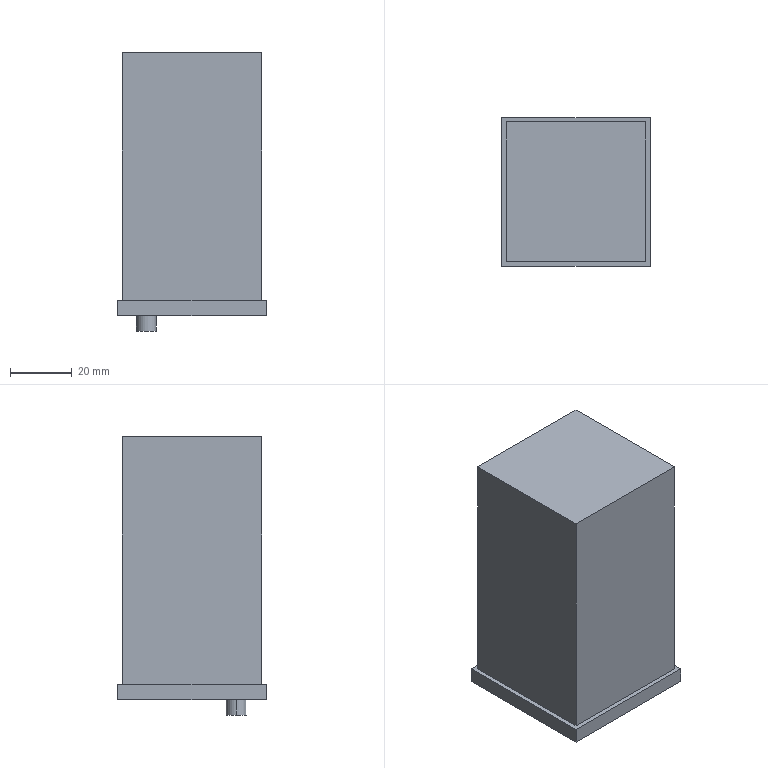Part | STEP file | Magnetic powder tension controller | 1 solid | 19 faces | box 48 x 48 x 90 mm | volume 173670 mm3 | plane 17 | cylinder 2 | commonest cylinder face diameters 6.473 x2
STEP:
#1=CARTESIAN_POINT('',(-17.962,-14.294,-5.));
#2=VERTEX_POINT('',#1);
#3=CARTESIAN_POINT('',(-11.489,-14.294,-5.));
#4=VERTEX_POINT('',#3);
#5=CARTESIAN_POINT('',(-14.726,-14.294,-5.));
#6=DIRECTION('',(0.,0.,-1.));
#7=DIRECTION('',(-1.,0.,0.));
#8=AXIS2_PLACEMENT_3D('',#5,#6,#7);
#9=CIRCLE('',#8,3.237);
#10=EDGE_CURVE('',#2,#4,#9,.T.);
#11=ORIENTED_EDGE('',*,*,#10,.F.);
#12=CARTESIAN_POINT('',(-17.962,-14.294,0.));
#13=VERTEX_POINT('',#12);
#14=CARTESIAN_POINT('',(-17.962,-14.294,-5.));
#15=DIRECTION('',(0.,0.,1.));
#16=VECTOR('',#15,1000.);
#17=LINE('',#14,#16);
#18=EDGE_CURVE('',#2,#13,#17,.T.);
#19=ORIENTED_EDGE('',*,*,#18,.T.);
#20=CARTESIAN_POINT('',(-11.489,-14.294,0.));
#21=VERTEX_POINT('',#20);
#22=CARTESIAN_POINT('',(-14.726,-14.294,0.));
#23=DIRECTION('',(0.,0.,-1.));
#24=DIRECTION('',(1.,0.,0.));
#25=AXIS2_PLACEMENT_3D('',#22,#23,#24);
#26=CIRCLE('',#25,3.237);
#27=EDGE_CURVE('',#13,#21,#26,.T.);
#28=ORIENTED_EDGE('',*,*,#27,.T.);
#29=CARTESIAN_POINT('',(-11.489,-14.294,-5.));
#30=DIRECTION('',(0.,0.,1.));
#31=VECTOR('',#30,1000.);
#32=LINE('',#29,#31);
#33=EDGE_CURVE('',#4,#21,#32,.T.);
#34=ORIENTED_EDGE('',*,*,#33,.F.);
#35=EDGE_LOOP('',(#11,#19,#28,#34));
#36=FACE_OUTER_BOUND('',#35,.T.);
#37=CARTESIAN_POINT('',(-14.726,-14.294,-5.));
#38=DIRECTION('',(0.,0.,1.));
#39=DIRECTION('',(1.,0.,0.));
#40=AXIS2_PLACEMENT_3D('',#37,#38,#39);
#41=CYLINDRICAL_SURFACE('',#40,3.237);
#42=ADVANCED_FACE('',(#36),#41,.T.);
#43=CARTESIAN_POINT('',(-24.,24.,0.));
#44=VERTEX_POINT('',#43);
#45=CARTESIAN_POINT('',(-24.,-24.,0.));
#46=VERTEX_POINT('',#45);
#47=CARTESIAN_POINT('',(-24.,-24.,0.));
#48=DIRECTION('',(0.,-1.,0.));
#49=VECTOR('',#48,1000.);
#50=LINE('',#47,#49);
#51=EDGE_CURVE('',#44,#46,#50,.T.);
#52=ORIENTED_EDGE('',*,*,#51,.T.);
#53=CARTESIAN_POINT('',(-24.,-24.,5.));
#54=VERTEX_POINT('',#53);
#55=CARTESIAN_POINT('',(-24.,-24.,5.));
#56=DIRECTION('',(0.,0.,-1.));
#57=VECTOR('',#56,1000.);
#58=LINE('',#55,#57);
#59=EDGE_CURVE('',#54,#46,#58,.T.);
#60=ORIENTED_EDGE('',*,*,#59,.F.);
#61=CARTESIAN_POINT('',(-24.,24.,5.));
#62=VERTEX_POINT('',#61);
#63=CARTESIAN_POINT('',(-24.,-24.,5.));
#64=DIRECTION('',(0.,-1.,0.));
#65=VECTOR('',#64,1000.);
#66=LINE('',#63,#65);
#67=EDGE_CURVE('',#62,#54,#66,.T.);
#68=ORIENTED_EDGE('',*,*,#67,.F.);
#69=CARTESIAN_POINT('',(-24.,24.,5.));
#70=DIRECTION('',(0.,0.,-1.));
#71=VECTOR('',#70,1000.);
#72=LINE('',#69,#71);
#73=EDGE_CURVE('',#62,#44,#72,.T.);
#74=ORIENTED_EDGE('',*,*,#73,.T.);
#75=EDGE_LOOP('',(#52,#60,#68,#74));
#76=FACE_OUTER_BOUND('',#75,.T.);
#77=CARTESIAN_POINT('',(-24.,-24.,5.));
#78=DIRECTION('',(1.,0.,0.));
#79=DIRECTION('',(0.,0.,-1.));
#80=AXIS2_PLACEMENT_3D('',#77,#78,#79);
#81=PLANE('',#80);
#82=ADVANCED_FACE('',(#76),#81,.F.);
#83=CARTESIAN_POINT('',(24.,-24.,0.));
#84=VERTEX_POINT('',#83);
#85=CARTESIAN_POINT('',(24.,-24.,0.));
#86=DIRECTION('',(1.,0.,0.));
#87=VECTOR('',#86,1000.);
#88=LINE('',#85,#87);
#89=EDGE_CURVE('',#46,#84,#88,.T.);
#90=ORIENTED_EDGE('',*,*,#89,.T.);
#91=CARTESIAN_POINT('',(24.,-24.,5.));
#92=VERTEX_POINT('',#91);
#93=CARTESIAN_POINT('',(24.,-24.,5.));
#94=DIRECTION('',(0.,0.,-1.));
#95=VECTOR('',#94,1000.);
#96=LINE('',#93,#95);
#97=EDGE_CURVE('',#92,#84,#96,.T.);
#98=ORIENTED_EDGE('',*,*,#97,.F.);
#99=CARTESIAN_POINT('',(24.,-24.,5.));
#100=DIRECTION('',(1.,0.,0.));
#101=VECTOR('',#100,1000.);
#102=LINE('',#99,#101);
#103=EDGE_CURVE('',#54,#92,#102,.T.);
#104=ORIENTED_EDGE('',*,*,#103,.F.);
#105=ORIENTED_EDGE('',*,*,#59,.T.);
#106=EDGE_LOOP('',(#90,#98,#104,#105));
#107=FACE_OUTER_BOUND('',#106,.T.);
#108=CARTESIAN_POINT('',(24.,-24.,5.));
#109=DIRECTION('',(0.,1.,0.));
#110=DIRECTION('',(0.,0.,1.));
#111=AXIS2_PLACEMENT_3D('',#108,#109,#110);
#112=PLANE('',#111);
#113=ADVANCED_FACE('',(#107),#112,.F.);
#114=CARTESIAN_POINT('',(24.,24.,0.));
#115=VERTEX_POINT('',#114);
#116=CARTESIAN_POINT('',(24.,-24.,0.));
#117=DIRECTION('',(0.,1.,0.));
#118=VECTOR('',#117,1000.);
#119=LINE('',#116,#118);
#120=EDGE_CURVE('',#84,#115,#119,.T.);
#121=ORIENTED_EDGE('',*,*,#120,.T.);
#122=CARTESIAN_POINT('',(24.,24.,5.));
#123=VERTEX_POINT('',#122);
#124=CARTESIAN_POINT('',(24.,24.,5.));
#125=DIRECTION('',(0.,0.,-1.));
#126=VECTOR('',#125,1000.);
#127=LINE('',#124,#126);
#128=EDGE_CURVE('',#123,#115,#127,.T.);
#129=ORIENTED_EDGE('',*,*,#128,.F.);
#130=CARTESIAN_POINT('',(24.,-24.,5.));
#131=DIRECTION('',(0.,1.,0.));
#132=VECTOR('',#131,1000.);
#133=LINE('',#130,#132);
#134=EDGE_CURVE('',#92,#123,#133,.T.);
#135=ORIENTED_EDGE('',*,*,#134,.F.);
#136=ORIENTED_EDGE('',*,*,#97,.T.);
#137=EDGE_LOOP('',(#121,#129,#135,#136));
#138=FACE_OUTER_BOUND('',#137,.T.);
#139=CARTESIAN_POINT('',(24.,-24.,5.));
#140=DIRECTION('',(-1.,0.,0.));
#141=DIRECTION('',(0.,0.,1.));
#142=AXIS2_PLACEMENT_3D('',#139,#140,#141);
#143=PLANE('',#142);
#144=ADVANCED_FACE('',(#138),#143,.F.);
#145=CARTESIAN_POINT('',(24.,24.,0.));
#146=DIRECTION('',(-1.,0.,0.));
#147=VECTOR('',#146,1000.);
#148=LINE('',#145,#147);
#149=EDGE_CURVE('',#115,#44,#148,.T.);
#150=ORIENTED_EDGE('',*,*,#149,.T.);
#151=ORIENTED_EDGE('',*,*,#73,.F.);
#152=CARTESIAN_POINT('',(24.,24.,5.));
#153=DIRECTION('',(-1.,0.,0.));
#154=VECTOR('',#153,1000.);
#155=LINE('',#152,#154);
#156=EDGE_CURVE('',#123,#62,#155,.T.);
#157=ORIENTED_EDGE('',*,*,#156,.F.);
#158=ORIENTED_EDGE('',*,*,#128,.T.);
#159=EDGE_LOOP('',(#150,#151,#157,#158));
#160=FACE_OUTER_BOUND('',#159,.T.);
#161=CARTESIAN_POINT('',(24.,24.,5.));
#162=DIRECTION('',(0.,-1.,0.));
#163=DIRECTION('',(0.,0.,-1.));
#164=AXIS2_PLACEMENT_3D('',#161,#162,#163);
#165=PLANE('',#164);
#166=ADVANCED_FACE('',(#160),#165,.F.);
#167=CARTESIAN_POINT('',(-22.5,22.5,5.));
#168=VERTEX_POINT('',#167);
#169=CARTESIAN_POINT('',(-22.5,-22.5,5.));
#170=VERTEX_POINT('',#169);
#171=CARTESIAN_POINT('',(-22.5,-22.5,5.));
#172=DIRECTION('',(0.,-1.,0.));
#173=VECTOR('',#172,1000.);
#174=LINE('',#171,#173);
#175=EDGE_CURVE('',#168,#170,#174,.T.);
#176=ORIENTED_EDGE('',*,*,#175,.F.);
#177=CARTESIAN_POINT('',(22.5,22.5,5.));
#178=VERTEX_POINT('',#177);
#179=CARTESIAN_POINT('',(22.5,22.5,5.));
#180=DIRECTION('',(-1.,0.,0.));
#181=VECTOR('',#180,1000.);
#182=LINE('',#179,#181);
#183=EDGE_CURVE('',#178,#168,#182,.T.);
#184=ORIENTED_EDGE('',*,*,#183,.F.);
#185=CARTESIAN_POINT('',(22.5,-22.5,5.));
#186=VERTEX_POINT('',#185);
#187=CARTESIAN_POINT('',(22.5,-22.5,5.));
#188=DIRECTION('',(0.,1.,0.));
#189=VECTOR('',#188,1000.);
#190=LINE('',#187,#189);
#191=EDGE_CURVE('',#186,#178,#190,.T.);
#192=ORIENTED_EDGE('',*,*,#191,.F.);
#193=CARTESIAN_POINT('',(22.5,-22.5,5.));
#194=DIRECTION('',(1.,0.,0.));
#195=VECTOR('',#194,1000.);
#196=LINE('',#193,#195);
#197=EDGE_CURVE('',#170,#186,#196,.T.);
#198=ORIENTED_EDGE('',*,*,#197,.F.);
#199=EDGE_LOOP('',(#176,#184,#192,#198));
#200=FACE_BOUND('',#199,.T.);
#201=ORIENTED_EDGE('',*,*,#67,.T.);
#202=ORIENTED_EDGE('',*,*,#103,.T.);
#203=ORIENTED_EDGE('',*,*,#134,.T.);
#204=ORIENTED_EDGE('',*,*,#156,.T.);
#205=EDGE_LOOP('',(#201,#202,#203,#204));
#206=FACE_OUTER_BOUND('',#205,.T.);
#207=CARTESIAN_POINT('',(0.,0.,5.));
#208=DIRECTION('',(0.,0.,1.));
#209=DIRECTION('',(1.,0.,0.));
#210=AXIS2_PLACEMENT_3D('',#207,#208,#209);
#211=PLANE('',#210);
#212=ADVANCED_FACE('',(#200,#206),#211,.T.);
#213=CARTESIAN_POINT('',(-14.726,-14.294,0.));
#214=DIRECTION('',(0.,0.,-1.));
#215=DIRECTION('',(1.,0.,0.));
#216=AXIS2_PLACEMENT_3D('',#213,#214,#215);
#217=CIRCLE('',#216,3.237);
#218=EDGE_CURVE('',#21,#13,#217,.T.);
#219=ORIENTED_EDGE('',*,*,#218,.F.);
#220=ORIENTED_EDGE('',*,*,#27,.F.);
#221=EDGE_LOOP('',(#219,#220));
#222=FACE_BOUND('',#221,.T.);
#223=CARTESIAN_POINT('',(-15.,17.5,0.));
#224=VERTEX_POINT('',#223);
#225=CARTESIAN_POINT('',(15.,17.5,0.));
#226=VERTEX_POINT('',#225);
#227=CARTESIAN_POINT('',(15.,17.5,0.));
#228=DIRECTION('',(1.,0.,0.));
#229=VECTOR('',#228,1000.);
#230=LINE('',#227,#229);
#231=EDGE_CURVE('',#224,#226,#230,.T.);
#232=ORIENTED_EDGE('',*,*,#231,.F.);
#233=CARTESIAN_POINT('',(-15.,12.5,0.));
#234=VERTEX_POINT('',#233);
#235=CARTESIAN_POINT('',(-15.,17.5,0.));
#236=DIRECTION('',(0.,1.,0.));
#237=VECTOR('',#236,1000.);
#238=LINE('',#235,#237);
#239=EDGE_CURVE('',#234,#224,#238,.T.);
#240=ORIENTED_EDGE('',*,*,#239,.F.);
#241=CARTESIAN_POINT('',(15.,12.5,0.));
#242=VERTEX_POINT('',#241);
#243=CARTESIAN_POINT('',(15.,12.5,0.));
#244=DIRECTION('',(-1.,0.,0.));
#245=VECTOR('',#244,1000.);
#246=LINE('',#243,#245);
#247=EDGE_CURVE('',#242,#234,#246,.T.);
#248=ORIENTED_EDGE('',*,*,#247,.F.);
#249=CARTESIAN_POINT('',(15.,17.5,0.));
#250=DIRECTION('',(0.,-1.,0.));
#251=VECTOR('',#250,1000.);
#252=LINE('',#249,#251);
#253=EDGE_CURVE('',#226,#242,#252,.T.);
#254=ORIENTED_EDGE('',*,*,#253,.F.);
#255=EDGE_LOOP('',(#232,#240,#248,#254));
#256=FACE_BOUND('',#255,.T.);
#257=ORIENTED_EDGE('',*,*,#51,.F.);
#258=ORIENTED_EDGE('',*,*,#149,.F.);
#259=ORIENTED_EDGE('',*,*,#120,.F.);
#260=ORIENTED_EDGE('',*,*,#89,.F.);
#261=EDGE_LOOP('',(#257,#258,#259,#260));
#262=FACE_OUTER_BOUND('',#261,.T.);
#263=CARTESIAN_POINT('',(0.,0.,0.));
#264=DIRECTION('',(0.,0.,1.));
#265=DIRECTION('',(1.,0.,0.));
#266=AXIS2_PLACEMENT_3D('',#263,#264,#265);
#267=PLANE('',#266);
#268=ADVANCED_FACE('',(#222,#256,#262),#267,.F.);
#269=ORIENTED_EDGE('',*,*,#175,.T.);
#270=CARTESIAN_POINT('',(-22.5,-22.5,85.));
#271=VERTEX_POINT('',#270);
#272=CARTESIAN_POINT('',(-22.5,-22.5,85.));
#273=DIRECTION('',(0.,0.,-1.));
#274=VECTOR('',#273,1000.);
#275=LINE('',#272,#274);
#276=EDGE_CURVE('',#271,#170,#275,.T.);
#277=ORIENTED_EDGE('',*,*,#276,.F.);
#278=CARTESIAN_POINT('',(-22.5,22.5,85.));
#279=VERTEX_POINT('',#278);
#280=CARTESIAN_POINT('',(-22.5,-22.5,85.));
#281=DIRECTION('',(0.,-1.,0.));
#282=VECTOR('',#281,1000.);
#283=LINE('',#280,#282);
#284=EDGE_CURVE('',#279,#271,#283,.T.);
#285=ORIENTED_EDGE('',*,*,#284,.F.);
#286=CARTESIAN_POINT('',(-22.5,22.5,85.));
#287=DIRECTION('',(0.,0.,-1.));
#288=VECTOR('',#287,1000.);
#289=LINE('',#286,#288);
#290=EDGE_CURVE('',#279,#168,#289,.T.);
#291=ORIENTED_EDGE('',*,*,#290,.T.);
#292=EDGE_LOOP('',(#269,#277,#285,#291));
#293=FACE_OUTER_BOUND('',#292,.T.);
#294=CARTESIAN_POINT('',(-22.5,-22.5,85.));
#295=DIRECTION('',(1.,0.,0.));
#296=DIRECTION('',(0.,0.,-1.));
#297=AXIS2_PLACEMENT_3D('',#294,#295,#296);
#298=PLANE('',#297);
#299=ADVANCED_FACE('',(#293),#298,.F.);
#300=ORIENTED_EDGE('',*,*,#197,.T.);
#301=CARTESIAN_POINT('',(22.5,-22.5,85.));
#302=VERTEX_POINT('',#301);
#303=CARTESIAN_POINT('',(22.5,-22.5,85.));
#304=DIRECTION('',(0.,0.,-1.));
#305=VECTOR('',#304,1000.);
#306=LINE('',#303,#305);
#307=EDGE_CURVE('',#302,#186,#306,.T.);
#308=ORIENTED_EDGE('',*,*,#307,.F.);
#309=CARTESIAN_POINT('',(22.5,-22.5,85.));
#310=DIRECTION('',(1.,0.,0.));
#311=VECTOR('',#310,1000.);
#312=LINE('',#309,#311);
#313=EDGE_CURVE('',#271,#302,#312,.T.);
#314=ORIENTED_EDGE('',*,*,#313,.F.);
#315=ORIENTED_EDGE('',*,*,#276,.T.);
#316=EDGE_LOOP('',(#300,#308,#314,#315));
#317=FACE_OUTER_BOUND('',#316,.T.);
#318=CARTESIAN_POINT('',(22.5,-22.5,85.));
#319=DIRECTION('',(0.,1.,0.));
#320=DIRECTION('',(0.,0.,1.));
#321=AXIS2_PLACEMENT_3D('',#318,#319,#320);
#322=PLANE('',#321);
#323=ADVANCED_FACE('',(#317),#322,.F.);
#324=ORIENTED_EDGE('',*,*,#191,.T.);
#325=CARTESIAN_POINT('',(22.5,22.5,85.));
#326=VERTEX_POINT('',#325);
#327=CARTESIAN_POINT('',(22.5,22.5,85.));
#328=DIRECTION('',(0.,0.,-1.));
#329=VECTOR('',#328,1000.);
#330=LINE('',#327,#329);
#331=EDGE_CURVE('',#326,#178,#330,.T.);
#332=ORIENTED_EDGE('',*,*,#331,.F.);
#333=CARTESIAN_POINT('',(22.5,-22.5,85.));
#334=DIRECTION('',(0.,1.,0.));
#335=VECTOR('',#334,1000.);
#336=LINE('',#333,#335);
#337=EDGE_CURVE('',#302,#326,#336,.T.);
#338=ORIENTED_EDGE('',*,*,#337,.F.);
#339=ORIENTED_EDGE('',*,*,#307,.T.);
#340=EDGE_LOOP('',(#324,#332,#338,#339));
#341=FACE_OUTER_BOUND('',#340,.T.);
#342=CARTESIAN_POINT('',(22.5,-22.5,85.));
#343=DIRECTION('',(-1.,0.,0.));
#344=DIRECTION('',(0.,0.,1.));
#345=AXIS2_PLACEMENT_3D('',#342,#343,#344);
#346=PLANE('',#345);
#347=ADVANCED_FACE('',(#341),#346,.F.);
#348=ORIENTED_EDGE('',*,*,#183,.T.);
#349=ORIENTED_EDGE('',*,*,#290,.F.);
#350=CARTESIAN_POINT('',(22.5,22.5,85.));
#351=DIRECTION('',(-1.,0.,0.));
#352=VECTOR('',#351,1000.);
#353=LINE('',#350,#352);
#354=EDGE_CURVE('',#326,#279,#353,.T.);
#355=ORIENTED_EDGE('',*,*,#354,.F.);
#356=ORIENTED_EDGE('',*,*,#331,.T.);
#357=EDGE_LOOP('',(#348,#349,#355,#356));
#358=FACE_OUTER_BOUND('',#357,.T.);
#359=CARTESIAN_POINT('',(22.5,22.5,85.));
#360=DIRECTION('',(0.,-1.,0.));
#361=DIRECTION('',(0.,0.,-1.));
#362=AXIS2_PLACEMENT_3D('',#359,#360,#361);
#363=PLANE('',#362);
#364=ADVANCED_FACE('',(#358),#363,.F.);
#365=ORIENTED_EDGE('',*,*,#284,.T.);
#366=ORIENTED_EDGE('',*,*,#313,.T.);
#367=ORIENTED_EDGE('',*,*,#337,.T.);
#368=ORIENTED_EDGE('',*,*,#354,.T.);
#369=EDGE_LOOP('',(#365,#366,#367,#368));
#370=FACE_OUTER_BOUND('',#369,.T.);
#371=CARTESIAN_POINT('',(0.,0.,85.));
#372=DIRECTION('',(0.,0.,1.));
#373=DIRECTION('',(1.,0.,0.));
#374=AXIS2_PLACEMENT_3D('',#371,#372,#373);
#375=PLANE('',#374);
#376=ADVANCED_FACE('',(#370),#375,.T.);
#377=ORIENTED_EDGE('',*,*,#239,.T.);
#378=CARTESIAN_POINT('',(-15.,17.5,0.1));
#379=VERTEX_POINT('',#378);
#380=CARTESIAN_POINT('',(-15.,17.5,0.1));
#381=DIRECTION('',(0.,0.,-1.));
#382=VECTOR('',#381,1000.);
#383=LINE('',#380,#382);
#384=EDGE_CURVE('',#379,#224,#383,.T.);
#385=ORIENTED_EDGE('',*,*,#384,.F.);
#386=CARTESIAN_POINT('',(-15.,12.5,0.1));
#387=VERTEX_POINT('',#386);
#388=CARTESIAN_POINT('',(-15.,17.5,0.1));
#389=DIRECTION('',(0.,1.,0.));
#390=VECTOR('',#389,1000.);
#391=LINE('',#388,#390);
#392=EDGE_CURVE('',#387,#379,#391,.T.);
#393=ORIENTED_EDGE('',*,*,#392,.F.);
#394=CARTESIAN_POINT('',(-15.,12.5,0.1));
#395=DIRECTION('',(0.,0.,-1.));
#396=VECTOR('',#395,1000.);
#397=LINE('',#394,#396);
#398=EDGE_CURVE('',#387,#234,#397,.T.);
#399=ORIENTED_EDGE('',*,*,#398,.T.);
#400=EDGE_LOOP('',(#377,#385,#393,#399));
#401=FACE_OUTER_BOUND('',#400,.T.);
#402=CARTESIAN_POINT('',(-15.,17.5,0.1));
#403=DIRECTION('',(-1.,0.,0.));
#404=DIRECTION('',(0.,0.,1.));
#405=AXIS2_PLACEMENT_3D('',#402,#403,#404);
#406=PLANE('',#405);
#407=ADVANCED_FACE('',(#401),#406,.F.);
#408=ORIENTED_EDGE('',*,*,#247,.T.);
#409=ORIENTED_EDGE('',*,*,#398,.F.);
#410=CARTESIAN_POINT('',(15.,12.5,0.1));
#411=VERTEX_POINT('',#410);
#412=CARTESIAN_POINT('',(15.,12.5,0.1));
#413=DIRECTION('',(-1.,0.,0.));
#414=VECTOR('',#413,1000.);
#415=LINE('',#412,#414);
#416=EDGE_CURVE('',#411,#387,#415,.T.);
#417=ORIENTED_EDGE('',*,*,#416,.F.);
#418=CARTESIAN_POINT('',(15.,12.5,0.1));
#419=DIRECTION('',(0.,0.,-1.));
#420=VECTOR('',#419,1000.);
#421=LINE('',#418,#420);
#422=EDGE_CURVE('',#411,#242,#421,.T.);
#423=ORIENTED_EDGE('',*,*,#422,.T.);
#424=EDGE_LOOP('',(#408,#409,#417,#423));
#425=FACE_OUTER_BOUND('',#424,.T.);
#426=CARTESIAN_POINT('',(15.,12.5,0.1));
#427=DIRECTION('',(0.,-1.,0.));
#428=DIRECTION('',(0.,0.,-1.));
#429=AXIS2_PLACEMENT_3D('',#426,#427,#428);
#430=PLANE('',#429);
#431=ADVANCED_FACE('',(#425),#430,.F.);
#432=ORIENTED_EDGE('',*,*,#253,.T.);
#433=ORIENTED_EDGE('',*,*,#422,.F.);
#434=CARTESIAN_POINT('',(15.,17.5,0.1));
#435=VERTEX_POINT('',#434);
#436=CARTESIAN_POINT('',(15.,17.5,0.1));
#437=DIRECTION('',(0.,-1.,0.));
#438=VECTOR('',#437,1000.);
#439=LINE('',#436,#438);
#440=EDGE_CURVE('',#435,#411,#439,.T.);
#441=ORIENTED_EDGE('',*,*,#440,.F.);
#442=CARTESIAN_POINT('',(15.,17.5,0.1));
#443=DIRECTION('',(0.,0.,-1.));
#444=VECTOR('',#443,1000.);
#445=LINE('',#442,#444);
#446=EDGE_CURVE('',#435,#226,#445,.T.);
#447=ORIENTED_EDGE('',*,*,#446,.T.);
#448=EDGE_LOOP('',(#432,#433,#441,#447));
#449=FACE_OUTER_BOUND('',#448,.T.);
#450=CARTESIAN_POINT('',(15.,17.5,0.1));
#451=DIRECTION('',(1.,0.,0.));
#452=DIRECTION('',(0.,0.,-1.));
#453=AXIS2_PLACEMENT_3D('',#450,#451,#452);
#454=PLANE('',#453);
#455=ADVANCED_FACE('',(#449),#454,.F.);
#456=ORIENTED_EDGE('',*,*,#231,.T.);
#457=ORIENTED_EDGE('',*,*,#446,.F.);
#458=CARTESIAN_POINT('',(15.,17.5,0.1));
#459=DIRECTION('',(1.,0.,0.));
#460=VECTOR('',#459,1000.);
#461=LINE('',#458,#460);
#462=EDGE_CURVE('',#379,#435,#461,.T.);
#463=ORIENTED_EDGE('',*,*,#462,.F.);
#464=ORIENTED_EDGE('',*,*,#384,.T.);
#465=EDGE_LOOP('',(#456,#457,#463,#464));
#466=FACE_OUTER_BOUND('',#465,.T.);
#467=CARTESIAN_POINT('',(15.,17.5,0.1));
#468=DIRECTION('',(0.,1.,0.));
#469=DIRECTION('',(-1.,0.,0.));
#470=AXIS2_PLACEMENT_3D('',#467,#468,#469);
#471=PLANE('',#470);
#472=ADVANCED_FACE('',(#466),#471,.F.);
#473=ORIENTED_EDGE('',*,*,#392,.T.);
#474=ORIENTED_EDGE('',*,*,#462,.T.);
#475=ORIENTED_EDGE('',*,*,#440,.T.);
#476=ORIENTED_EDGE('',*,*,#416,.T.);
#477=EDGE_LOOP('',(#473,#474,#475,#476));
#478=FACE_OUTER_BOUND('',#477,.T.);
#479=CARTESIAN_POINT('',(0.,0.,0.1));
#480=DIRECTION('',(0.,0.,-1.));
#481=DIRECTION('',(-1.,0.,0.));
#482=AXIS2_PLACEMENT_3D('',#479,#480,#481);
#483=PLANE('',#482);
#484=ADVANCED_FACE('',(#478),#483,.T.);
#485=ORIENTED_EDGE('',*,*,#18,.F.);
#486=CARTESIAN_POINT('',(-14.726,-14.294,-5.));
#487=DIRECTION('',(0.,0.,-1.));
#488=DIRECTION('',(-1.,0.,0.));
#489=AXIS2_PLACEMENT_3D('',#486,#487,#488);
#490=CIRCLE('',#489,3.237);
#491=EDGE_CURVE('',#4,#2,#490,.T.);
#492=ORIENTED_EDGE('',*,*,#491,.F.);
#493=ORIENTED_EDGE('',*,*,#33,.T.);
#494=ORIENTED_EDGE('',*,*,#218,.T.);
#495=EDGE_LOOP('',(#485,#492,#493,#494));
#496=FACE_OUTER_BOUND('',#495,.T.);
#497=CARTESIAN_POINT('',(-14.726,-14.294,-5.));
#498=DIRECTION('',(0.,0.,1.));
#499=DIRECTION('',(1.,0.,0.));
#500=AXIS2_PLACEMENT_3D('',#497,#498,#499);
#501=CYLINDRICAL_SURFACE('',#500,3.237);
#502=ADVANCED_FACE('',(#496),#501,.T.);
#503=ORIENTED_EDGE('',*,*,#491,.T.);
#504=ORIENTED_EDGE('',*,*,#10,.T.);
#505=EDGE_LOOP('',(#503,#504));
#506=FACE_OUTER_BOUND('',#505,.T.);
#507=CARTESIAN_POINT('',(-14.726,-14.294,-5.));
#508=DIRECTION('',(0.,0.,-1.));
#509=DIRECTION('',(-1.,0.,0.));
#510=AXIS2_PLACEMENT_3D('',#507,#508,#509);
#511=PLANE('',#510);
#512=ADVANCED_FACE('',(#506),#511,.T.);
#513=CLOSED_SHELL('',(#42,#82,#113,#144,#166,#212,#268,#299,#323,#347,#364,#376,#407,#431,#455,#472,#484,#502,#512));
#514=MANIFOLD_SOLID_BREP('',#513);
#515=CARTESIAN_POINT('',(0.,0.,0.));
#516=DIRECTION('',(0.,0.,1.));
#517=DIRECTION('',(1.,0.,0.));
#518=AXIS2_PLACEMENT_3D('',#515,#516,#517);
#519=(LENGTH_UNIT()NAMED_UNIT(*)SI_UNIT(.MILLI.,.METRE.));
#520=UNCERTAINTY_MEASURE_WITH_UNIT(LENGTH_MEASURE(0.00001),#519,'','');
#521=(NAMED_UNIT(*)PLANE_ANGLE_UNIT()SI_UNIT($,.RADIAN.));
#522=(NAMED_UNIT(*)SI_UNIT($,.STERADIAN.)SOLID_ANGLE_UNIT());
#523=(GEOMETRIC_REPRESENTATION_CONTEXT(3)GLOBAL_UNCERTAINTY_ASSIGNED_CONTEXT((#520))GLOBAL_UNIT_ASSIGNED_CONTEXT((#519,#521,#522))REPRESENTATION_CONTEXT('',''));
#524=ADVANCED_BREP_SHAPE_REPRESENTATION('',(#514,#518),#523);